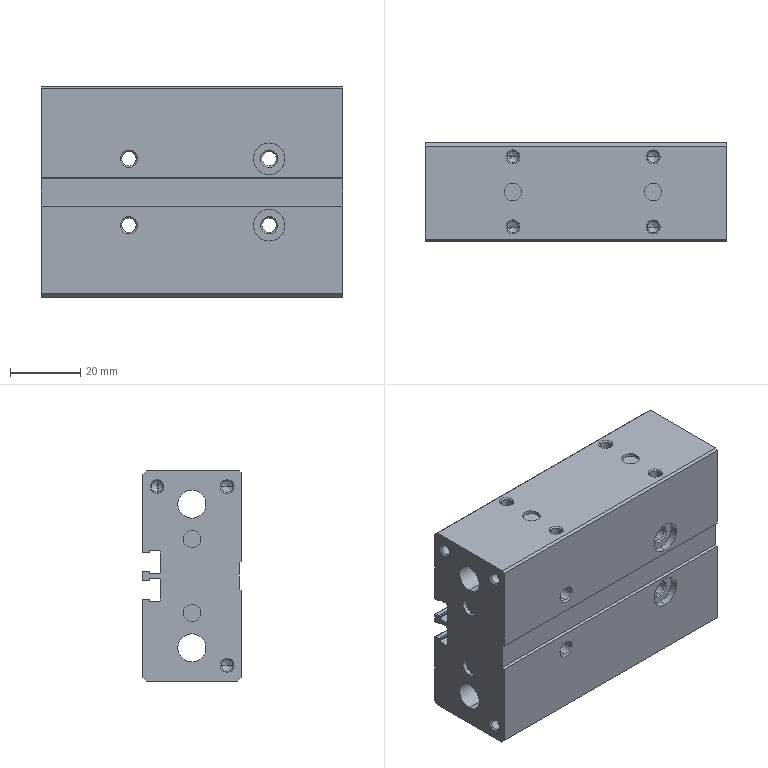Part | SolidWorks | features BaseBody 1 | 1 solid | 207 faces | box 86 x 28.05 x 60 mm | volume 119405 mm3 | cylinder 100 | plane 63 | cone 44 | commonest cylinder face diameters 0.4 x16 0.8 x16 4.134 x16 3.242 x14 8 x12 4.3 x8